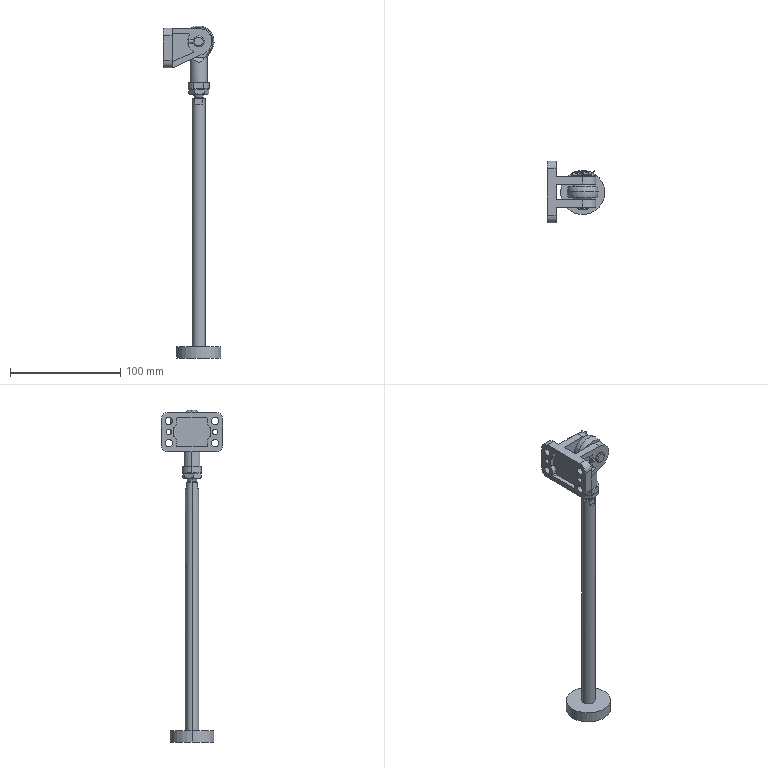Part | SolidWorks | features CompositeCurve 1 | 6 solids | 207 faces | box 52 x 56 x 300.673 mm | volume 74670 mm3 | cylinder 99 | plane 75 | cone 23 | sphere 6 | torus 4 | commonest cylinder face diameters 2 x22 10 x12 6.8 x8 14.8 x6 2.6 x4 3.6 x4